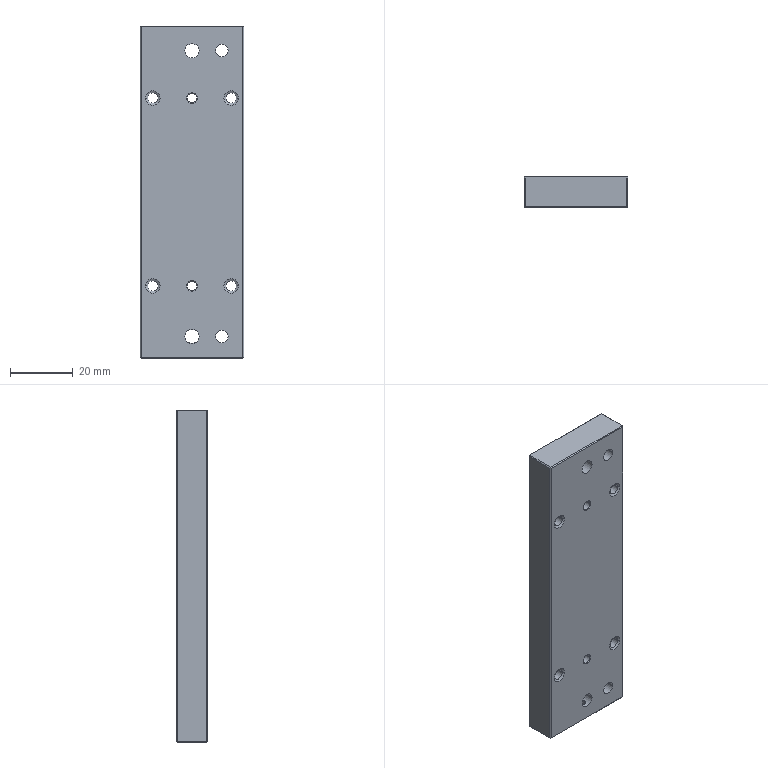Part | 1 solid | 70 faces | box 33 x 10 x 106 mm | volume 33560 mm3 | cylinder 30 | plane 20 | cone 20 | commonest cylinder face diameters 3.3 x8 2.5 x6 3 x4 4 x4 4.5 x4 8 x4